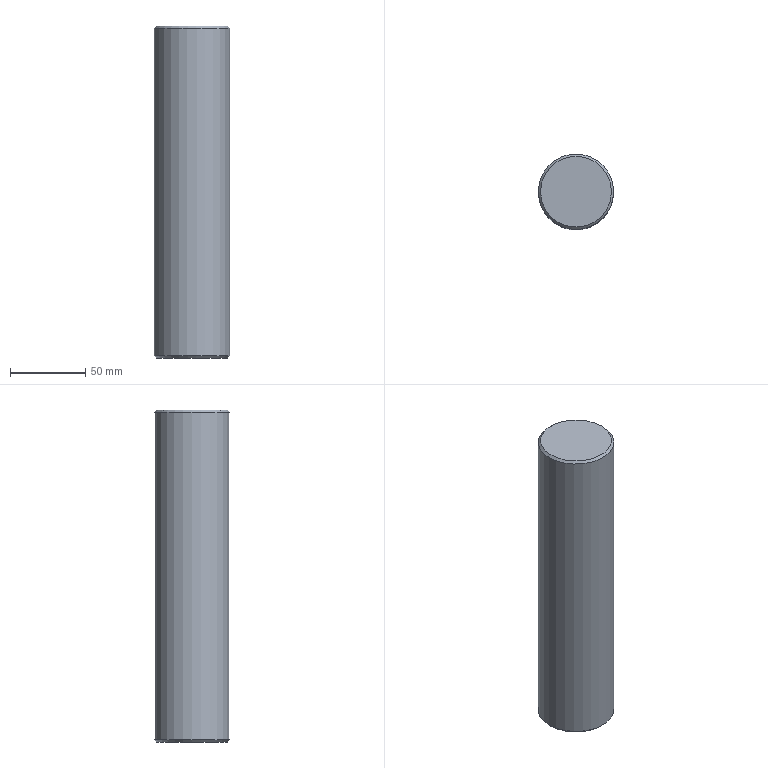Part | STEP file | solid 72 | 1 solid | 9 faces | box 50 x 50 x 220 mm | volume 430674 mm3 | plane 3 | cylinder 3 | cone 3 | commonest cylinder face diameters 6.7 x1 8 x1 50 x1